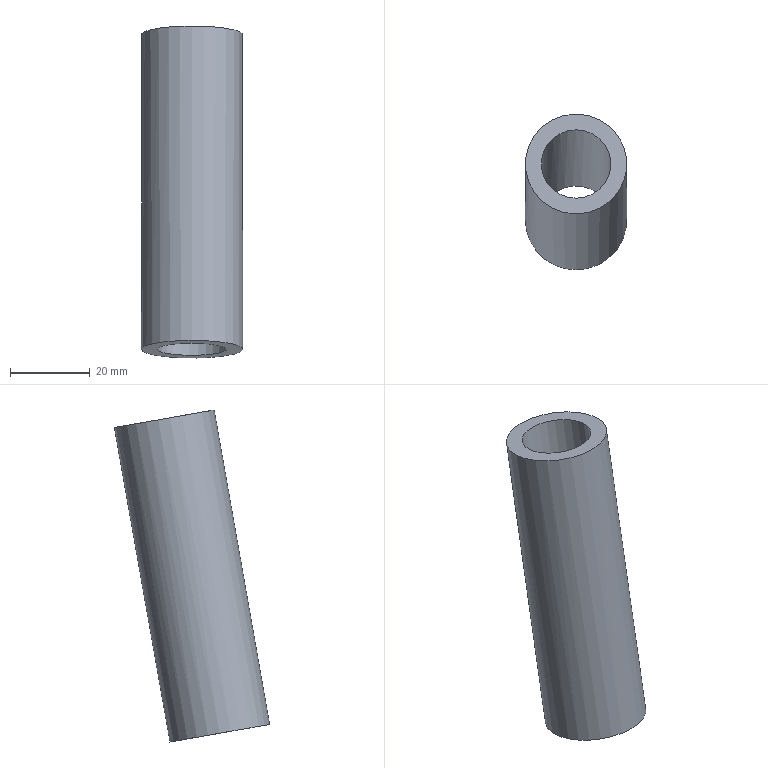Part | NX | features solid 2 | 1 solid | 4 faces | box 25.4 x 38.906 x 83.195 mm | volume 21514 mm3 | cylinder 2 | plane 2 | commonest cylinder face diameters 17.4 x1 25.4 x1
STEP:
#1=CARTESIAN_POINT('',(-1073.5,-836.47,140.931));
#2=VERTEX_POINT('',#1);
#3=CARTESIAN_POINT('',(-1073.5,-827.903,139.42));
#4=DIRECTION('',(0.,-0.1736,-0.9848));
#5=DIRECTION('',(0.,-0.9848,0.1736));
#6=AXIS2_PLACEMENT_3D('',#3,#4,#5);
#7=CIRCLE('',#6,8.7);
#8=EDGE_CURVE('',#2,#2,#7,.F.);
#9=ORIENTED_EDGE('',*,*,#8,.T.);
#10=EDGE_LOOP('',(#9));
#11=FACE_BOUND('',#10,.T.);
#12=CARTESIAN_POINT('',(-1082.2,-841.795,60.636));
#13=VERTEX_POINT('',#12);
#14=CARTESIAN_POINT('',(-1073.5,-841.795,60.636));
#15=DIRECTION('',(0.,0.1736,0.9848));
#16=DIRECTION('',(-1.,0.,0.));
#17=AXIS2_PLACEMENT_3D('',#14,#15,#16);
#18=CIRCLE('',#17,8.7);
#19=EDGE_CURVE('',#13,#13,#18,.T.);
#20=ORIENTED_EDGE('',*,*,#19,.F.);
#21=EDGE_LOOP('',(#20));
#22=FACE_BOUND('',#21,.T.);
#23=CARTESIAN_POINT('',(-1073.5,-819.22,188.661));
#24=DIRECTION('',(0.,-0.1736,-0.9848));
#25=DIRECTION('',(1.,0.,0.));
#26=AXIS2_PLACEMENT_3D('',#23,#24,#25);
#27=CYLINDRICAL_SURFACE('',#26,8.7);
#28=ADVANCED_FACE('',(#11,#22),#27,.F.);
#29=CARTESIAN_POINT('',(-1073.5,-840.41,141.626));
#30=VERTEX_POINT('',#29);
#31=CARTESIAN_POINT('',(-1073.5,-827.903,139.42));
#32=DIRECTION('',(0.,-0.1736,-0.9848));
#33=DIRECTION('',(0.,-0.9848,0.1736));
#34=AXIS2_PLACEMENT_3D('',#31,#32,#33);
#35=CIRCLE('',#34,12.7);
#36=EDGE_CURVE('',#30,#30,#35,.F.);
#37=ORIENTED_EDGE('',*,*,#36,.F.);
#38=EDGE_LOOP('',(#37));
#39=FACE_BOUND('',#38,.T.);
#40=CARTESIAN_POINT('',(-1086.2,-841.795,60.636));
#41=VERTEX_POINT('',#40);
#42=CARTESIAN_POINT('',(-1073.5,-841.795,60.636));
#43=DIRECTION('',(0.,0.1736,0.9848));
#44=DIRECTION('',(-1.,0.,0.));
#45=AXIS2_PLACEMENT_3D('',#42,#43,#44);
#46=CIRCLE('',#45,12.7);
#47=EDGE_CURVE('',#41,#41,#46,.T.);
#48=ORIENTED_EDGE('',*,*,#47,.T.);
#49=EDGE_LOOP('',(#48));
#50=FACE_BOUND('',#49,.T.);
#51=CARTESIAN_POINT('',(-1073.5,-819.22,188.661));
#52=DIRECTION('',(0.,-0.1736,-0.9848));
#53=DIRECTION('',(1.,0.,0.));
#54=AXIS2_PLACEMENT_3D('',#51,#52,#53);
#55=CYLINDRICAL_SURFACE('',#54,12.7);
#56=ADVANCED_FACE('',(#39,#50),#55,.T.);
#57=ORIENTED_EDGE('',*,*,#8,.F.);
#58=EDGE_LOOP('',(#57));
#59=FACE_BOUND('',#58,.T.);
#60=ORIENTED_EDGE('',*,*,#36,.T.);
#61=EDGE_LOOP('',(#60));
#62=FACE_BOUND('',#61,.T.);
#63=CARTESIAN_POINT('',(-1073.5,-827.903,139.42));
#64=DIRECTION('',(0.,0.1736,0.9848));
#65=DIRECTION('',(-1.,0.,0.));
#66=AXIS2_PLACEMENT_3D('',#63,#64,#65);
#67=PLANE('',#66);
#68=ADVANCED_FACE('',(#59,#62),#67,.T.);
#69=ORIENTED_EDGE('',*,*,#19,.T.);
#70=EDGE_LOOP('',(#69));
#71=FACE_BOUND('',#70,.T.);
#72=ORIENTED_EDGE('',*,*,#47,.F.);
#73=EDGE_LOOP('',(#72));
#74=FACE_BOUND('',#73,.T.);
#75=CARTESIAN_POINT('',(-1073.5,-841.795,60.636));
#76=DIRECTION('',(0.,0.1736,0.9848));
#77=DIRECTION('',(-1.,0.,0.));
#78=AXIS2_PLACEMENT_3D('',#75,#76,#77);
#79=PLANE('',#78);
#80=ADVANCED_FACE('',(#71,#74),#79,.F.);
#81=CLOSED_SHELL('',(#28,#56,#68,#80));
#82=MANIFOLD_SOLID_BREP('',#81);
#83=(LENGTH_UNIT()NAMED_UNIT(*)SI_UNIT(.MILLI.,.METRE.));
#84=UNCERTAINTY_MEASURE_WITH_UNIT(LENGTH_MEASURE(0.00001),#83,'','');
#85=(NAMED_UNIT(*)PLANE_ANGLE_UNIT()SI_UNIT($,.RADIAN.));
#86=(NAMED_UNIT(*)SI_UNIT($,.STERADIAN.)SOLID_ANGLE_UNIT());
#87=(GEOMETRIC_REPRESENTATION_CONTEXT(3)GLOBAL_UNCERTAINTY_ASSIGNED_CONTEXT((#84))GLOBAL_UNIT_ASSIGNED_CONTEXT((#83,#85,#86))REPRESENTATION_CONTEXT('',''));
#88=ADVANCED_BREP_SHAPE_REPRESENTATION('',(#82),#87);